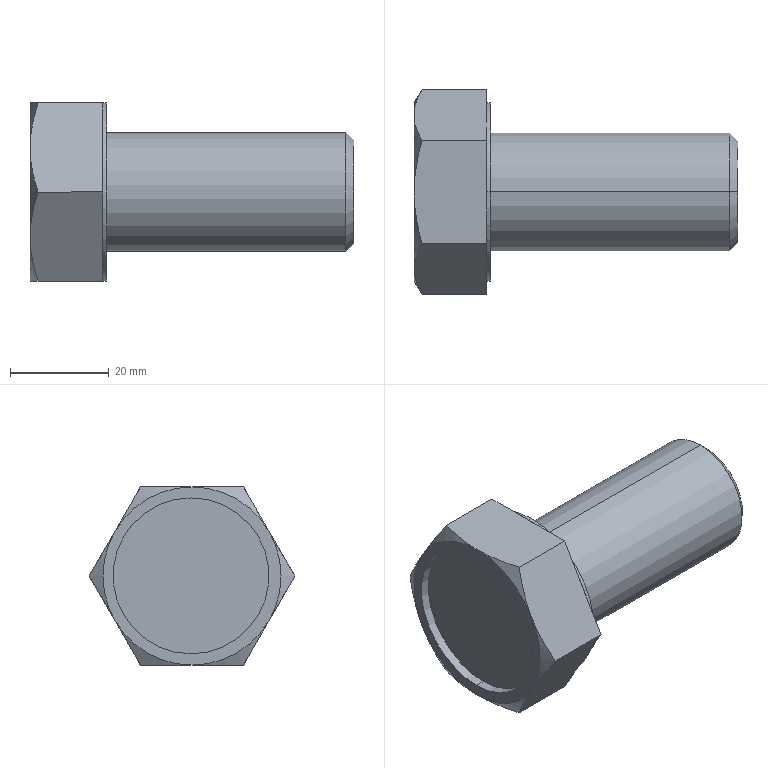Part | STEP file | formed hex screw_am_B18.2.3.2M - Formed hex screw, M24 x 3.0 x 50 --50WN | 1 solid | 30 faces | box 65.44 x 41.569 x 36 mm | volume 38213 mm3 | plane 16 | cone 8 | cylinder 6 | commonest cylinder face diameters 24 x2 31.5 x2 36 x2